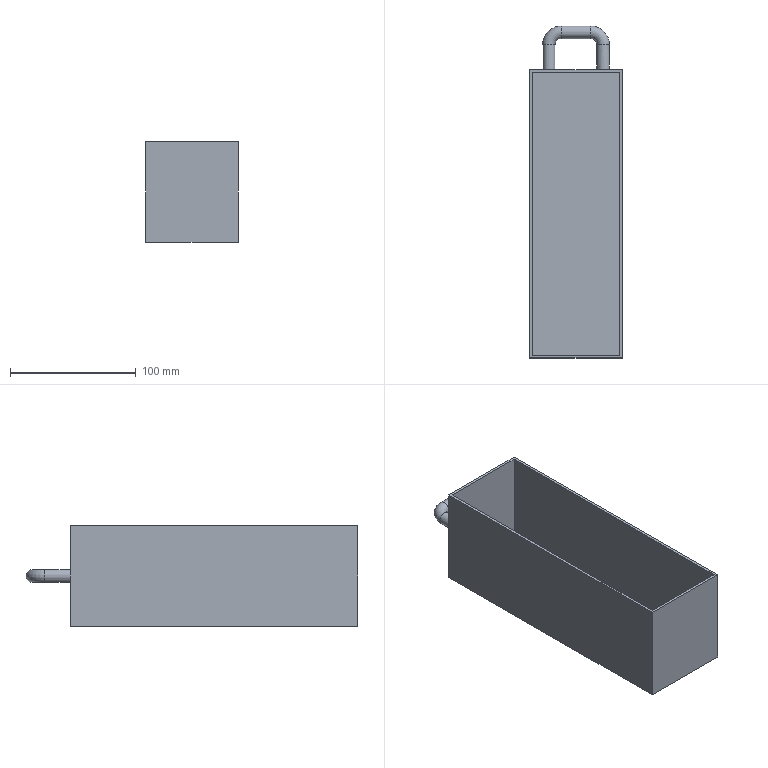Part | NX | features solid 2 | 1 solid | 16 faces | box 73.493 x 263.569 x 80 mm | volume 134017 mm3 | plane 11 | cylinder 3 | torus 2 | commonest cylinder face diameters 10 x3
STEP:
#1=CARTESIAN_POINT('',(100.,500.,-253.));
#2=VERTEX_POINT('',#1);
#3=CARTESIAN_POINT('',(100.,500.,-258.));
#4=DIRECTION('',(0.,1.,0.));
#5=DIRECTION('',(0.,0.,1.));
#6=AXIS2_PLACEMENT_3D('',#3,#4,#5);
#7=CIRCLE('',#6,5.);
#8=EDGE_CURVE('',#2,#2,#7,.T.);
#9=ORIENTED_EDGE('',*,*,#8,.F.);
#10=EDGE_LOOP('',(#9));
#11=FACE_BOUND('',#10,.T.);
#12=CARTESIAN_POINT('',(158.306,500.,-218.));
#13=VERTEX_POINT('',#12);
#14=CARTESIAN_POINT('',(84.813,500.,-218.));
#15=VERTEX_POINT('',#14);
#16=CARTESIAN_POINT('',(340.,500.,-218.));
#17=DIRECTION('',(-1.,0.,0.));
#18=VECTOR('',#17,1000.);
#19=LINE('',#16,#18);
#20=EDGE_CURVE('',#13,#15,#19,.T.);
#21=ORIENTED_EDGE('',*,*,#20,.F.);
#22=CARTESIAN_POINT('',(158.306,500.,-298.));
#23=VERTEX_POINT('',#22);
#24=CARTESIAN_POINT('',(158.306,500.,-188.));
#25=DIRECTION('',(0.,0.,1.));
#26=VECTOR('',#25,1000.);
#27=LINE('',#24,#26);
#28=EDGE_CURVE('',#23,#13,#27,.T.);
#29=ORIENTED_EDGE('',*,*,#28,.F.);
#30=CARTESIAN_POINT('',(84.813,500.,-298.));
#31=VERTEX_POINT('',#30);
#32=CARTESIAN_POINT('',(340.,500.,-298.));
#33=DIRECTION('',(-1.,0.,0.));
#34=VECTOR('',#33,1000.);
#35=LINE('',#32,#34);
#36=EDGE_CURVE('',#23,#31,#35,.T.);
#37=ORIENTED_EDGE('',*,*,#36,.T.);
#38=CARTESIAN_POINT('',(84.813,500.,-298.));
#39=DIRECTION('',(0.,0.,1.));
#40=VECTOR('',#39,1000.);
#41=LINE('',#38,#40);
#42=EDGE_CURVE('',#31,#15,#41,.T.);
#43=ORIENTED_EDGE('',*,*,#42,.T.);
#44=EDGE_LOOP('',(#21,#29,#37,#43));
#45=FACE_BOUND('',#44,.T.);
#46=CARTESIAN_POINT('',(138.119,500.,-258.));
#47=VERTEX_POINT('',#46);
#48=CARTESIAN_POINT('',(143.119,500.,-258.));
#49=DIRECTION('',(0.,1.,0.));
#50=DIRECTION('',(-1.,0.,0.));
#51=AXIS2_PLACEMENT_3D('',#48,#49,#50);
#52=CIRCLE('',#51,5.);
#53=EDGE_CURVE('',#47,#47,#52,.F.);
#54=ORIENTED_EDGE('',*,*,#53,.T.);
#55=EDGE_LOOP('',(#54));
#56=FACE_BOUND('',#55,.T.);
#57=CARTESIAN_POINT('',(340.,500.,-188.));
#58=DIRECTION('',(0.,-1.,0.));
#59=DIRECTION('',(-1.,0.,0.));
#60=AXIS2_PLACEMENT_3D('',#57,#58,#59);
#61=PLANE('',#60);
#62=ADVANCED_FACE('',(#11,#45,#56),#61,.F.);
#63=CARTESIAN_POINT('',(84.813,271.431,-218.));
#64=VERTEX_POINT('',#63);
#65=CARTESIAN_POINT('',(158.306,271.431,-218.));
#66=VERTEX_POINT('',#65);
#67=CARTESIAN_POINT('',(84.813,271.431,-218.));
#68=DIRECTION('',(1.,0.,0.));
#69=VECTOR('',#68,1000.);
#70=LINE('',#67,#69);
#71=EDGE_CURVE('',#64,#66,#70,.T.);
#72=ORIENTED_EDGE('',*,*,#71,.F.);
#73=CARTESIAN_POINT('',(84.813,271.431,-298.));
#74=VERTEX_POINT('',#73);
#75=CARTESIAN_POINT('',(84.813,271.431,-298.));
#76=DIRECTION('',(0.,0.,1.));
#77=VECTOR('',#76,1000.);
#78=LINE('',#75,#77);
#79=EDGE_CURVE('',#74,#64,#78,.T.);
#80=ORIENTED_EDGE('',*,*,#79,.F.);
#81=CARTESIAN_POINT('',(158.306,271.431,-298.));
#82=VERTEX_POINT('',#81);
#83=CARTESIAN_POINT('',(84.813,271.431,-298.));
#84=DIRECTION('',(1.,0.,0.));
#85=VECTOR('',#84,1000.);
#86=LINE('',#83,#85);
#87=EDGE_CURVE('',#74,#82,#86,.T.);
#88=ORIENTED_EDGE('',*,*,#87,.T.);
#89=CARTESIAN_POINT('',(158.306,271.431,-298.));
#90=DIRECTION('',(0.,0.,1.));
#91=VECTOR('',#90,1000.);
#92=LINE('',#89,#91);
#93=EDGE_CURVE('',#82,#66,#92,.T.);
#94=ORIENTED_EDGE('',*,*,#93,.T.);
#95=EDGE_LOOP('',(#72,#80,#88,#94));
#96=FACE_BOUND('',#95,.T.);
#97=CARTESIAN_POINT('',(84.813,271.431,-298.));
#98=DIRECTION('',(0.,1.,0.));
#99=DIRECTION('',(0.,0.,1.));
#100=AXIS2_PLACEMENT_3D('',#97,#98,#99);
#101=PLANE('',#100);
#102=ADVANCED_FACE('',(#96),#101,.F.);
#103=CARTESIAN_POINT('',(158.306,311.431,-218.));
#104=DIRECTION('',(0.,1.,0.));
#105=VECTOR('',#104,1000.);
#106=LINE('',#103,#105);
#107=EDGE_CURVE('',#66,#13,#106,.T.);
#108=ORIENTED_EDGE('',*,*,#107,.F.);
#109=ORIENTED_EDGE('',*,*,#93,.F.);
#110=CARTESIAN_POINT('',(158.306,311.431,-298.));
#111=DIRECTION('',(0.,1.,0.));
#112=VECTOR('',#111,1000.);
#113=LINE('',#110,#112);
#114=EDGE_CURVE('',#82,#23,#113,.T.);
#115=ORIENTED_EDGE('',*,*,#114,.T.);
#116=ORIENTED_EDGE('',*,*,#28,.T.);
#117=EDGE_LOOP('',(#108,#109,#115,#116));
#118=FACE_BOUND('',#117,.T.);
#119=CARTESIAN_POINT('',(158.306,311.431,-298.));
#120=DIRECTION('',(-1.,0.,0.));
#121=DIRECTION('',(0.,0.,-1.));
#122=AXIS2_PLACEMENT_3D('',#119,#120,#121);
#123=PLANE('',#122);
#124=ADVANCED_FACE('',(#118),#123,.F.);
#125=CARTESIAN_POINT('',(84.813,500.89,-218.));
#126=DIRECTION('',(0.,-1.,0.));
#127=VECTOR('',#126,1000.);
#128=LINE('',#125,#127);
#129=EDGE_CURVE('',#15,#64,#128,.T.);
#130=ORIENTED_EDGE('',*,*,#129,.F.);
#131=ORIENTED_EDGE('',*,*,#42,.F.);
#132=CARTESIAN_POINT('',(84.813,500.89,-298.));
#133=DIRECTION('',(0.,-1.,0.));
#134=VECTOR('',#133,1000.);
#135=LINE('',#132,#134);
#136=EDGE_CURVE('',#31,#74,#135,.T.);
#137=ORIENTED_EDGE('',*,*,#136,.T.);
#138=ORIENTED_EDGE('',*,*,#79,.T.);
#139=EDGE_LOOP('',(#130,#131,#137,#138));
#140=FACE_BOUND('',#139,.T.);
#141=CARTESIAN_POINT('',(84.813,500.89,-298.));
#142=DIRECTION('',(1.,0.,0.));
#143=DIRECTION('',(0.,0.,1.));
#144=AXIS2_PLACEMENT_3D('',#141,#142,#143);
#145=PLANE('',#144);
#146=ADVANCED_FACE('',(#140),#145,.F.);
#147=ORIENTED_EDGE('',*,*,#87,.F.);
#148=ORIENTED_EDGE('',*,*,#136,.F.);
#149=ORIENTED_EDGE('',*,*,#36,.F.);
#150=ORIENTED_EDGE('',*,*,#114,.F.);
#151=EDGE_LOOP('',(#147,#148,#149,#150));
#152=FACE_BOUND('',#151,.T.);
#153=CARTESIAN_POINT('',(158.306,311.431,-298.));
#154=DIRECTION('',(0.,0.,-1.));
#155=DIRECTION('',(1.,0.,0.));
#156=AXIS2_PLACEMENT_3D('',#153,#154,#155);
#157=PLANE('',#156);
#158=ADVANCED_FACE('',(#152),#157,.T.);
#159=CARTESIAN_POINT('',(86.813,498.,-218.));
#160=VERTEX_POINT('',#159);
#161=CARTESIAN_POINT('',(86.813,273.431,-218.));
#162=VERTEX_POINT('',#161);
#163=CARTESIAN_POINT('',(86.813,500.89,-218.));
#164=DIRECTION('',(0.,-1.,0.));
#165=VECTOR('',#164,1000.);
#166=LINE('',#163,#165);
#167=EDGE_CURVE('',#160,#162,#166,.T.);
#168=ORIENTED_EDGE('',*,*,#167,.F.);
#169=CARTESIAN_POINT('',(156.306,498.,-218.));
#170=VERTEX_POINT('',#169);
#171=CARTESIAN_POINT('',(340.,498.,-218.));
#172=DIRECTION('',(-1.,0.,0.));
#173=VECTOR('',#172,1000.);
#174=LINE('',#171,#173);
#175=EDGE_CURVE('',#170,#160,#174,.T.);
#176=ORIENTED_EDGE('',*,*,#175,.F.);
#177=CARTESIAN_POINT('',(156.306,273.431,-218.));
#178=VERTEX_POINT('',#177);
#179=CARTESIAN_POINT('',(156.306,311.431,-218.));
#180=DIRECTION('',(0.,1.,0.));
#181=VECTOR('',#180,1000.);
#182=LINE('',#179,#181);
#183=EDGE_CURVE('',#178,#170,#182,.T.);
#184=ORIENTED_EDGE('',*,*,#183,.F.);
#185=CARTESIAN_POINT('',(84.813,273.431,-218.));
#186=DIRECTION('',(1.,0.,0.));
#187=VECTOR('',#186,1000.);
#188=LINE('',#185,#187);
#189=EDGE_CURVE('',#162,#178,#188,.T.);
#190=ORIENTED_EDGE('',*,*,#189,.F.);
#191=EDGE_LOOP('',(#168,#176,#184,#190));
#192=FACE_BOUND('',#191,.T.);
#193=ORIENTED_EDGE('',*,*,#71,.T.);
#194=ORIENTED_EDGE('',*,*,#107,.T.);
#195=ORIENTED_EDGE('',*,*,#20,.T.);
#196=ORIENTED_EDGE('',*,*,#129,.T.);
#197=EDGE_LOOP('',(#193,#194,#195,#196));
#198=FACE_BOUND('',#197,.T.);
#199=CARTESIAN_POINT('',(158.306,311.431,-218.));
#200=DIRECTION('',(0.,0.,-1.));
#201=DIRECTION('',(1.,0.,0.));
#202=AXIS2_PLACEMENT_3D('',#199,#200,#201);
#203=PLANE('',#202);
#204=ADVANCED_FACE('',(#192,#198),#203,.F.);
#205=ORIENTED_EDGE('',*,*,#189,.T.);
#206=CARTESIAN_POINT('',(156.306,273.431,-296.));
#207=VERTEX_POINT('',#206);
#208=CARTESIAN_POINT('',(156.306,273.431,-298.));
#209=DIRECTION('',(0.,0.,1.));
#210=VECTOR('',#209,1000.);
#211=LINE('',#208,#210);
#212=EDGE_CURVE('',#207,#178,#211,.T.);
#213=ORIENTED_EDGE('',*,*,#212,.F.);
#214=CARTESIAN_POINT('',(86.813,273.431,-296.));
#215=VERTEX_POINT('',#214);
#216=CARTESIAN_POINT('',(84.813,273.431,-296.));
#217=DIRECTION('',(1.,0.,0.));
#218=VECTOR('',#217,1000.);
#219=LINE('',#216,#218);
#220=EDGE_CURVE('',#215,#207,#219,.T.);
#221=ORIENTED_EDGE('',*,*,#220,.F.);
#222=CARTESIAN_POINT('',(86.813,273.431,-298.));
#223=DIRECTION('',(0.,0.,1.));
#224=VECTOR('',#223,1000.);
#225=LINE('',#222,#224);
#226=EDGE_CURVE('',#215,#162,#225,.T.);
#227=ORIENTED_EDGE('',*,*,#226,.T.);
#228=EDGE_LOOP('',(#205,#213,#221,#227));
#229=FACE_BOUND('',#228,.T.);
#230=CARTESIAN_POINT('',(84.813,273.431,-298.));
#231=DIRECTION('',(0.,1.,0.));
#232=DIRECTION('',(0.,0.,1.));
#233=AXIS2_PLACEMENT_3D('',#230,#231,#232);
#234=PLANE('',#233);
#235=ADVANCED_FACE('',(#229),#234,.T.);
#236=ORIENTED_EDGE('',*,*,#183,.T.);
#237=CARTESIAN_POINT('',(156.306,498.,-296.));
#238=VERTEX_POINT('',#237);
#239=CARTESIAN_POINT('',(156.306,498.,-188.));
#240=DIRECTION('',(0.,0.,1.));
#241=VECTOR('',#240,1000.);
#242=LINE('',#239,#241);
#243=EDGE_CURVE('',#238,#170,#242,.T.);
#244=ORIENTED_EDGE('',*,*,#243,.F.);
#245=CARTESIAN_POINT('',(156.306,311.431,-296.));
#246=DIRECTION('',(0.,1.,0.));
#247=VECTOR('',#246,1000.);
#248=LINE('',#245,#247);
#249=EDGE_CURVE('',#207,#238,#248,.T.);
#250=ORIENTED_EDGE('',*,*,#249,.F.);
#251=ORIENTED_EDGE('',*,*,#212,.T.);
#252=EDGE_LOOP('',(#236,#244,#250,#251));
#253=FACE_BOUND('',#252,.T.);
#254=CARTESIAN_POINT('',(156.306,311.431,-298.));
#255=DIRECTION('',(-1.,0.,0.));
#256=DIRECTION('',(0.,0.,-1.));
#257=AXIS2_PLACEMENT_3D('',#254,#255,#256);
#258=PLANE('',#257);
#259=ADVANCED_FACE('',(#253),#258,.T.);
#260=ORIENTED_EDGE('',*,*,#175,.T.);
#261=CARTESIAN_POINT('',(86.813,498.,-296.));
#262=VERTEX_POINT('',#261);
#263=CARTESIAN_POINT('',(86.813,498.,-298.));
#264=DIRECTION('',(0.,0.,1.));
#265=VECTOR('',#264,1000.);
#266=LINE('',#263,#265);
#267=EDGE_CURVE('',#262,#160,#266,.T.);
#268=ORIENTED_EDGE('',*,*,#267,.F.);
#269=CARTESIAN_POINT('',(340.,498.,-296.));
#270=DIRECTION('',(-1.,0.,0.));
#271=VECTOR('',#270,1000.);
#272=LINE('',#269,#271);
#273=EDGE_CURVE('',#238,#262,#272,.T.);
#274=ORIENTED_EDGE('',*,*,#273,.F.);
#275=ORIENTED_EDGE('',*,*,#243,.T.);
#276=EDGE_LOOP('',(#260,#268,#274,#275));
#277=FACE_BOUND('',#276,.T.);
#278=CARTESIAN_POINT('',(340.,498.,-188.));
#279=DIRECTION('',(0.,-1.,0.));
#280=DIRECTION('',(-1.,0.,0.));
#281=AXIS2_PLACEMENT_3D('',#278,#279,#280);
#282=PLANE('',#281);
#283=ADVANCED_FACE('',(#277),#282,.T.);
#284=ORIENTED_EDGE('',*,*,#167,.T.);
#285=ORIENTED_EDGE('',*,*,#226,.F.);
#286=CARTESIAN_POINT('',(86.813,500.89,-296.));
#287=DIRECTION('',(0.,-1.,0.));
#288=VECTOR('',#287,1000.);
#289=LINE('',#286,#288);
#290=EDGE_CURVE('',#262,#215,#289,.T.);
#291=ORIENTED_EDGE('',*,*,#290,.F.);
#292=ORIENTED_EDGE('',*,*,#267,.T.);
#293=EDGE_LOOP('',(#284,#285,#291,#292));
#294=FACE_BOUND('',#293,.T.);
#295=CARTESIAN_POINT('',(86.813,500.89,-298.));
#296=DIRECTION('',(1.,0.,0.));
#297=DIRECTION('',(0.,0.,1.));
#298=AXIS2_PLACEMENT_3D('',#295,#296,#297);
#299=PLANE('',#298);
#300=ADVANCED_FACE('',(#294),#299,.T.);
#301=ORIENTED_EDGE('',*,*,#220,.T.);
#302=ORIENTED_EDGE('',*,*,#249,.T.);
#303=ORIENTED_EDGE('',*,*,#273,.T.);
#304=ORIENTED_EDGE('',*,*,#290,.T.);
#305=EDGE_LOOP('',(#301,#302,#303,#304));
#306=FACE_BOUND('',#305,.T.);
#307=CARTESIAN_POINT('',(158.306,311.431,-296.));
#308=DIRECTION('',(0.,0.,-1.));
#309=DIRECTION('',(1.,0.,0.));
#310=AXIS2_PLACEMENT_3D('',#307,#308,#309);
#311=PLANE('',#310);
#312=ADVANCED_FACE('',(#306),#311,.F.);
#313=CARTESIAN_POINT('',(100.,520.,-253.));
#314=VERTEX_POINT('',#313);
#315=CARTESIAN_POINT('',(100.,520.,-258.));
#316=DIRECTION('',(0.,1.,0.));
#317=DIRECTION('',(0.,0.,1.));
#318=AXIS2_PLACEMENT_3D('',#315,#316,#317);
#319=CIRCLE('',#318,5.);
#320=EDGE_CURVE('',#314,#314,#319,.T.);
#321=ORIENTED_EDGE('',*,*,#320,.F.);
#322=EDGE_LOOP('',(#321));
#323=FACE_BOUND('',#322,.T.);
#324=ORIENTED_EDGE('',*,*,#8,.T.);
#325=EDGE_LOOP('',(#324));
#326=FACE_BOUND('',#325,.T.);
#327=CARTESIAN_POINT('',(100.,520.,-258.));
#328=DIRECTION('',(0.,-1.,0.));
#329=DIRECTION('',(0.,0.,-1.));
#330=AXIS2_PLACEMENT_3D('',#327,#328,#329);
#331=CYLINDRICAL_SURFACE('',#330,5.);
#332=ADVANCED_FACE('',(#323,#326),#331,.T.);
#333=CARTESIAN_POINT('',(110.,530.,-253.));
#334=VERTEX_POINT('',#333);
#335=CARTESIAN_POINT('',(110.,530.,-258.));
#336=DIRECTION('',(1.,0.,0.));
#337=DIRECTION('',(0.,0.,1.));
#338=AXIS2_PLACEMENT_3D('',#335,#336,#337);
#339=CIRCLE('',#338,5.);
#340=EDGE_CURVE('',#334,#334,#339,.T.);
#341=ORIENTED_EDGE('',*,*,#340,.F.);
#342=EDGE_LOOP('',(#341));
#343=FACE_BOUND('',#342,.T.);
#344=ORIENTED_EDGE('',*,*,#320,.T.);
#345=EDGE_LOOP('',(#344));
#346=FACE_BOUND('',#345,.T.);
#347=CARTESIAN_POINT('',(110.,520.,-258.));
#348=DIRECTION('',(0.,0.,-1.));
#349=DIRECTION('',(1.,0.,0.));
#350=AXIS2_PLACEMENT_3D('',#347,#348,#349);
#351=TOROIDAL_SURFACE('',#350,10.,5.);
#352=ADVANCED_FACE('',(#343,#346),#351,.T.);
#353=CARTESIAN_POINT('',(133.119,530.,-253.));
#354=VERTEX_POINT('',#353);
#355=CARTESIAN_POINT('',(133.119,530.,-258.));
#356=DIRECTION('',(1.,0.,0.));
#357=DIRECTION('',(0.,0.,1.));
#358=AXIS2_PLACEMENT_3D('',#355,#356,#357);
#359=CIRCLE('',#358,5.);
#360=EDGE_CURVE('',#354,#354,#359,.T.);
#361=ORIENTED_EDGE('',*,*,#360,.F.);
#362=EDGE_LOOP('',(#361));
#363=FACE_BOUND('',#362,.T.);
#364=ORIENTED_EDGE('',*,*,#340,.T.);
#365=EDGE_LOOP('',(#364));
#366=FACE_BOUND('',#365,.T.);
#367=CARTESIAN_POINT('',(133.119,530.,-258.));
#368=DIRECTION('',(-1.,0.,0.));
#369=DIRECTION('',(0.,0.,-1.));
#370=AXIS2_PLACEMENT_3D('',#367,#368,#369);
#371=CYLINDRICAL_SURFACE('',#370,5.);
#372=ADVANCED_FACE('',(#363,#366),#371,.T.);
#373=CARTESIAN_POINT('',(143.119,520.,-253.));
#374=VERTEX_POINT('',#373);
#375=CARTESIAN_POINT('',(143.119,520.,-258.));
#376=DIRECTION('',(0.,-1.,0.));
#377=DIRECTION('',(0.,0.,1.));
#378=AXIS2_PLACEMENT_3D('',#375,#376,#377);
#379=CIRCLE('',#378,5.);
#380=EDGE_CURVE('',#374,#374,#379,.T.);
#381=ORIENTED_EDGE('',*,*,#380,.F.);
#382=EDGE_LOOP('',(#381));
#383=FACE_BOUND('',#382,.T.);
#384=ORIENTED_EDGE('',*,*,#360,.T.);
#385=EDGE_LOOP('',(#384));
#386=FACE_BOUND('',#385,.T.);
#387=CARTESIAN_POINT('',(133.119,520.,-258.));
#388=DIRECTION('',(0.,0.,-1.));
#389=DIRECTION('',(1.,0.,0.));
#390=AXIS2_PLACEMENT_3D('',#387,#388,#389);
#391=TOROIDAL_SURFACE('',#390,10.,5.);
#392=ADVANCED_FACE('',(#383,#386),#391,.T.);
#393=ORIENTED_EDGE('',*,*,#380,.T.);
#394=EDGE_LOOP('',(#393));
#395=FACE_BOUND('',#394,.T.);
#396=ORIENTED_EDGE('',*,*,#53,.F.);
#397=EDGE_LOOP('',(#396));
#398=FACE_BOUND('',#397,.T.);
#399=CARTESIAN_POINT('',(143.119,520.,-258.));
#400=DIRECTION('',(0.,-1.,0.));
#401=DIRECTION('',(0.,0.,-1.));
#402=AXIS2_PLACEMENT_3D('',#399,#400,#401);
#403=CYLINDRICAL_SURFACE('',#402,5.);
#404=ADVANCED_FACE('',(#395,#398),#403,.T.);
#405=CLOSED_SHELL('',(#62,#102,#124,#146,#158,#204,#235,#259,#283,#300,#312,#332,#352,#372,#392,#404));
#406=MANIFOLD_SOLID_BREP('',#405);
#407=(LENGTH_UNIT()NAMED_UNIT(*)SI_UNIT(.MILLI.,.METRE.));
#408=UNCERTAINTY_MEASURE_WITH_UNIT(LENGTH_MEASURE(0.00001),#407,'','');
#409=(NAMED_UNIT(*)PLANE_ANGLE_UNIT()SI_UNIT($,.RADIAN.));
#410=(NAMED_UNIT(*)SI_UNIT($,.STERADIAN.)SOLID_ANGLE_UNIT());
#411=(GEOMETRIC_REPRESENTATION_CONTEXT(3)GLOBAL_UNCERTAINTY_ASSIGNED_CONTEXT((#408))GLOBAL_UNIT_ASSIGNED_CONTEXT((#407,#409,#410))REPRESENTATION_CONTEXT('',''));
#412=ADVANCED_BREP_SHAPE_REPRESENTATION('',(#406),#411);